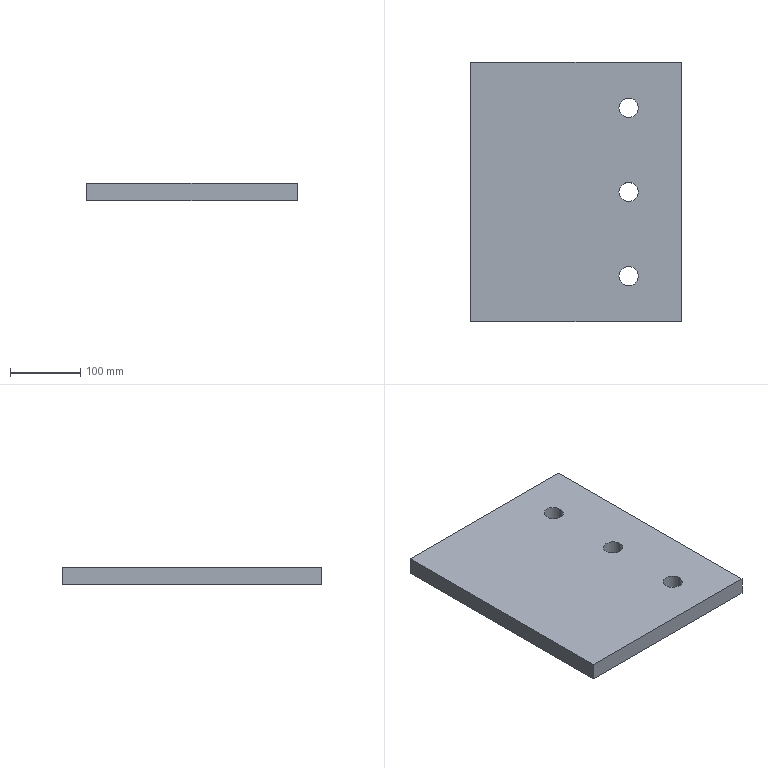Part | SolidWorks | features Extrusion 1 | 1 solid | 12 faces | box 300 x 370 x 25 mm | volume 2730453 mm3 | cylinder 6 | plane 6 | commonest cylinder face diameters 27.5 x6
STEP:
#1=CARTESIAN_POINT('',(211.25,65.,25.));
#2=VERTEX_POINT('',#1);
#3=CARTESIAN_POINT('',(238.75,65.,25.));
#4=VERTEX_POINT('',#3);
#5=CARTESIAN_POINT('',(225.,65.,25.));
#6=DIRECTION('',(0.,0.,1.));
#7=DIRECTION('',(1.,0.,0.));
#8=AXIS2_PLACEMENT_3D('',#5,#6,#7);
#9=CIRCLE('',#8,13.75);
#10=EDGE_CURVE('',#2,#4,#9,.T.);
#11=ORIENTED_EDGE('',*,*,#10,.T.);
#12=CARTESIAN_POINT('',(238.75,65.,0.));
#13=VERTEX_POINT('',#12);
#14=CARTESIAN_POINT('',(238.75,65.,25.));
#15=DIRECTION('',(0.,0.,-1.));
#16=VECTOR('',#15,1000.);
#17=LINE('',#14,#16);
#18=EDGE_CURVE('',#4,#13,#17,.T.);
#19=ORIENTED_EDGE('',*,*,#18,.T.);
#20=CARTESIAN_POINT('',(211.25,65.,0.));
#21=VERTEX_POINT('',#20);
#22=CARTESIAN_POINT('',(225.,65.,0.));
#23=DIRECTION('',(0.,0.,1.));
#24=DIRECTION('',(1.,0.,0.));
#25=AXIS2_PLACEMENT_3D('',#22,#23,#24);
#26=CIRCLE('',#25,13.75);
#27=EDGE_CURVE('',#21,#13,#26,.T.);
#28=ORIENTED_EDGE('',*,*,#27,.F.);
#29=CARTESIAN_POINT('',(211.25,65.,25.));
#30=DIRECTION('',(0.,0.,-1.));
#31=VECTOR('',#30,1000.);
#32=LINE('',#29,#31);
#33=EDGE_CURVE('',#2,#21,#32,.T.);
#34=ORIENTED_EDGE('',*,*,#33,.F.);
#35=EDGE_LOOP('',(#11,#19,#28,#34));
#36=FACE_OUTER_BOUND('',#35,.T.);
#37=CARTESIAN_POINT('',(225.,65.,25.));
#38=DIRECTION('',(0.,0.,-1.));
#39=DIRECTION('',(-1.,0.,0.));
#40=AXIS2_PLACEMENT_3D('',#37,#38,#39);
#41=CYLINDRICAL_SURFACE('',#40,13.75);
#42=ADVANCED_FACE('',(#36),#41,.F.);
#43=CARTESIAN_POINT('',(211.25,185.,25.));
#44=VERTEX_POINT('',#43);
#45=CARTESIAN_POINT('',(238.75,185.,25.));
#46=VERTEX_POINT('',#45);
#47=CARTESIAN_POINT('',(225.,185.,25.));
#48=DIRECTION('',(0.,0.,1.));
#49=DIRECTION('',(1.,0.,0.));
#50=AXIS2_PLACEMENT_3D('',#47,#48,#49);
#51=CIRCLE('',#50,13.75);
#52=EDGE_CURVE('',#44,#46,#51,.T.);
#53=ORIENTED_EDGE('',*,*,#52,.T.);
#54=CARTESIAN_POINT('',(238.75,185.,0.));
#55=VERTEX_POINT('',#54);
#56=CARTESIAN_POINT('',(238.75,185.,25.));
#57=DIRECTION('',(0.,0.,-1.));
#58=VECTOR('',#57,1000.);
#59=LINE('',#56,#58);
#60=EDGE_CURVE('',#46,#55,#59,.T.);
#61=ORIENTED_EDGE('',*,*,#60,.T.);
#62=CARTESIAN_POINT('',(211.25,185.,0.));
#63=VERTEX_POINT('',#62);
#64=CARTESIAN_POINT('',(225.,185.,0.));
#65=DIRECTION('',(0.,0.,1.));
#66=DIRECTION('',(1.,0.,0.));
#67=AXIS2_PLACEMENT_3D('',#64,#65,#66);
#68=CIRCLE('',#67,13.75);
#69=EDGE_CURVE('',#63,#55,#68,.T.);
#70=ORIENTED_EDGE('',*,*,#69,.F.);
#71=CARTESIAN_POINT('',(211.25,185.,25.));
#72=DIRECTION('',(0.,0.,-1.));
#73=VECTOR('',#72,1000.);
#74=LINE('',#71,#73);
#75=EDGE_CURVE('',#44,#63,#74,.T.);
#76=ORIENTED_EDGE('',*,*,#75,.F.);
#77=EDGE_LOOP('',(#53,#61,#70,#76));
#78=FACE_OUTER_BOUND('',#77,.T.);
#79=CARTESIAN_POINT('',(225.,185.,25.));
#80=DIRECTION('',(0.,0.,-1.));
#81=DIRECTION('',(-1.,0.,0.));
#82=AXIS2_PLACEMENT_3D('',#79,#80,#81);
#83=CYLINDRICAL_SURFACE('',#82,13.75);
#84=ADVANCED_FACE('',(#78),#83,.F.);
#85=CARTESIAN_POINT('',(211.25,305.,25.));
#86=VERTEX_POINT('',#85);
#87=CARTESIAN_POINT('',(238.75,305.,25.));
#88=VERTEX_POINT('',#87);
#89=CARTESIAN_POINT('',(225.,305.,25.));
#90=DIRECTION('',(0.,0.,1.));
#91=DIRECTION('',(1.,0.,0.));
#92=AXIS2_PLACEMENT_3D('',#89,#90,#91);
#93=CIRCLE('',#92,13.75);
#94=EDGE_CURVE('',#86,#88,#93,.T.);
#95=ORIENTED_EDGE('',*,*,#94,.T.);
#96=CARTESIAN_POINT('',(238.75,305.,0.));
#97=VERTEX_POINT('',#96);
#98=CARTESIAN_POINT('',(238.75,305.,25.));
#99=DIRECTION('',(0.,0.,-1.));
#100=VECTOR('',#99,1000.);
#101=LINE('',#98,#100);
#102=EDGE_CURVE('',#88,#97,#101,.T.);
#103=ORIENTED_EDGE('',*,*,#102,.T.);
#104=CARTESIAN_POINT('',(211.25,305.,0.));
#105=VERTEX_POINT('',#104);
#106=CARTESIAN_POINT('',(225.,305.,0.));
#107=DIRECTION('',(0.,0.,1.));
#108=DIRECTION('',(1.,0.,0.));
#109=AXIS2_PLACEMENT_3D('',#106,#107,#108);
#110=CIRCLE('',#109,13.75);
#111=EDGE_CURVE('',#105,#97,#110,.T.);
#112=ORIENTED_EDGE('',*,*,#111,.F.);
#113=CARTESIAN_POINT('',(211.25,305.,25.));
#114=DIRECTION('',(0.,0.,-1.));
#115=VECTOR('',#114,1000.);
#116=LINE('',#113,#115);
#117=EDGE_CURVE('',#86,#105,#116,.T.);
#118=ORIENTED_EDGE('',*,*,#117,.F.);
#119=EDGE_LOOP('',(#95,#103,#112,#118));
#120=FACE_OUTER_BOUND('',#119,.T.);
#121=CARTESIAN_POINT('',(225.,305.,25.));
#122=DIRECTION('',(0.,0.,-1.));
#123=DIRECTION('',(-1.,0.,0.));
#124=AXIS2_PLACEMENT_3D('',#121,#122,#123);
#125=CYLINDRICAL_SURFACE('',#124,13.75);
#126=ADVANCED_FACE('',(#120),#125,.F.);
#127=CARTESIAN_POINT('',(0.,370.,25.));
#128=VERTEX_POINT('',#127);
#129=CARTESIAN_POINT('',(0.,0.,25.));
#130=VERTEX_POINT('',#129);
#131=CARTESIAN_POINT('',(0.,0.,25.));
#132=DIRECTION('',(0.,-1.,0.));
#133=VECTOR('',#132,1000.);
#134=LINE('',#131,#133);
#135=EDGE_CURVE('',#128,#130,#134,.T.);
#136=ORIENTED_EDGE('',*,*,#135,.T.);
#137=CARTESIAN_POINT('',(300.,0.,25.));
#138=VERTEX_POINT('',#137);
#139=CARTESIAN_POINT('',(0.,0.,25.));
#140=DIRECTION('',(1.,0.,0.));
#141=VECTOR('',#140,1000.);
#142=LINE('',#139,#141);
#143=EDGE_CURVE('',#130,#138,#142,.T.);
#144=ORIENTED_EDGE('',*,*,#143,.T.);
#145=CARTESIAN_POINT('',(300.,370.,25.));
#146=VERTEX_POINT('',#145);
#147=CARTESIAN_POINT('',(300.,0.,25.));
#148=DIRECTION('',(0.,1.,0.));
#149=VECTOR('',#148,1000.);
#150=LINE('',#147,#149);
#151=EDGE_CURVE('',#138,#146,#150,.T.);
#152=ORIENTED_EDGE('',*,*,#151,.T.);
#153=CARTESIAN_POINT('',(0.,370.,25.));
#154=DIRECTION('',(-1.,0.,0.));
#155=VECTOR('',#154,1000.);
#156=LINE('',#153,#155);
#157=EDGE_CURVE('',#146,#128,#156,.T.);
#158=ORIENTED_EDGE('',*,*,#157,.T.);
#159=EDGE_LOOP('',(#136,#144,#152,#158));
#160=FACE_OUTER_BOUND('',#159,.T.);
#161=ORIENTED_EDGE('',*,*,#94,.F.);
#162=CARTESIAN_POINT('',(225.,305.,25.));
#163=DIRECTION('',(0.,0.,1.));
#164=DIRECTION('',(1.,0.,0.));
#165=AXIS2_PLACEMENT_3D('',#162,#163,#164);
#166=CIRCLE('',#165,13.75);
#167=EDGE_CURVE('',#88,#86,#166,.T.);
#168=ORIENTED_EDGE('',*,*,#167,.F.);
#169=EDGE_LOOP('',(#161,#168));
#170=FACE_BOUND('',#169,.T.);
#171=ORIENTED_EDGE('',*,*,#52,.F.);
#172=CARTESIAN_POINT('',(225.,185.,25.));
#173=DIRECTION('',(0.,0.,1.));
#174=DIRECTION('',(1.,0.,0.));
#175=AXIS2_PLACEMENT_3D('',#172,#173,#174);
#176=CIRCLE('',#175,13.75);
#177=EDGE_CURVE('',#46,#44,#176,.T.);
#178=ORIENTED_EDGE('',*,*,#177,.F.);
#179=EDGE_LOOP('',(#171,#178));
#180=FACE_BOUND('',#179,.T.);
#181=ORIENTED_EDGE('',*,*,#10,.F.);
#182=CARTESIAN_POINT('',(225.,65.,25.));
#183=DIRECTION('',(0.,0.,1.));
#184=DIRECTION('',(1.,0.,0.));
#185=AXIS2_PLACEMENT_3D('',#182,#183,#184);
#186=CIRCLE('',#185,13.75);
#187=EDGE_CURVE('',#4,#2,#186,.T.);
#188=ORIENTED_EDGE('',*,*,#187,.F.);
#189=EDGE_LOOP('',(#181,#188));
#190=FACE_BOUND('',#189,.T.);
#191=CARTESIAN_POINT('',(0.,0.,25.));
#192=DIRECTION('',(0.,0.,-1.));
#193=DIRECTION('',(-1.,0.,0.));
#194=AXIS2_PLACEMENT_3D('',#191,#192,#193);
#195=PLANE('',#194);
#196=ADVANCED_FACE('',(#160,#170,#180,#190),#195,.F.);
#197=ORIENTED_EDGE('',*,*,#69,.T.);
#198=CARTESIAN_POINT('',(225.,185.,0.));
#199=DIRECTION('',(0.,0.,1.));
#200=DIRECTION('',(1.,0.,0.));
#201=AXIS2_PLACEMENT_3D('',#198,#199,#200);
#202=CIRCLE('',#201,13.75);
#203=EDGE_CURVE('',#55,#63,#202,.T.);
#204=ORIENTED_EDGE('',*,*,#203,.T.);
#205=EDGE_LOOP('',(#197,#204));
#206=FACE_BOUND('',#205,.T.);
#207=CARTESIAN_POINT('',(0.,370.,0.));
#208=VERTEX_POINT('',#207);
#209=CARTESIAN_POINT('',(0.,0.,0.));
#210=VERTEX_POINT('',#209);
#211=CARTESIAN_POINT('',(0.,0.,0.));
#212=DIRECTION('',(0.,-1.,0.));
#213=VECTOR('',#212,1000.);
#214=LINE('',#211,#213);
#215=EDGE_CURVE('',#208,#210,#214,.T.);
#216=ORIENTED_EDGE('',*,*,#215,.F.);
#217=CARTESIAN_POINT('',(300.,370.,0.));
#218=VERTEX_POINT('',#217);
#219=CARTESIAN_POINT('',(0.,370.,0.));
#220=DIRECTION('',(-1.,0.,0.));
#221=VECTOR('',#220,1000.);
#222=LINE('',#219,#221);
#223=EDGE_CURVE('',#218,#208,#222,.T.);
#224=ORIENTED_EDGE('',*,*,#223,.F.);
#225=CARTESIAN_POINT('',(300.,0.,0.));
#226=VERTEX_POINT('',#225);
#227=CARTESIAN_POINT('',(300.,0.,0.));
#228=DIRECTION('',(0.,1.,0.));
#229=VECTOR('',#228,1000.);
#230=LINE('',#227,#229);
#231=EDGE_CURVE('',#226,#218,#230,.T.);
#232=ORIENTED_EDGE('',*,*,#231,.F.);
#233=CARTESIAN_POINT('',(0.,0.,0.));
#234=DIRECTION('',(1.,0.,0.));
#235=VECTOR('',#234,1000.);
#236=LINE('',#233,#235);
#237=EDGE_CURVE('',#210,#226,#236,.T.);
#238=ORIENTED_EDGE('',*,*,#237,.F.);
#239=EDGE_LOOP('',(#216,#224,#232,#238));
#240=FACE_OUTER_BOUND('',#239,.T.);
#241=ORIENTED_EDGE('',*,*,#111,.T.);
#242=CARTESIAN_POINT('',(225.,305.,0.));
#243=DIRECTION('',(0.,0.,1.));
#244=DIRECTION('',(1.,0.,0.));
#245=AXIS2_PLACEMENT_3D('',#242,#243,#244);
#246=CIRCLE('',#245,13.75);
#247=EDGE_CURVE('',#97,#105,#246,.T.);
#248=ORIENTED_EDGE('',*,*,#247,.T.);
#249=EDGE_LOOP('',(#241,#248));
#250=FACE_BOUND('',#249,.T.);
#251=ORIENTED_EDGE('',*,*,#27,.T.);
#252=CARTESIAN_POINT('',(225.,65.,0.));
#253=DIRECTION('',(0.,0.,1.));
#254=DIRECTION('',(1.,0.,0.));
#255=AXIS2_PLACEMENT_3D('',#252,#253,#254);
#256=CIRCLE('',#255,13.75);
#257=EDGE_CURVE('',#13,#21,#256,.T.);
#258=ORIENTED_EDGE('',*,*,#257,.T.);
#259=EDGE_LOOP('',(#251,#258));
#260=FACE_BOUND('',#259,.T.);
#261=CARTESIAN_POINT('',(0.,0.,0.));
#262=DIRECTION('',(0.,0.,-1.));
#263=DIRECTION('',(-1.,0.,0.));
#264=AXIS2_PLACEMENT_3D('',#261,#262,#263);
#265=PLANE('',#264);
#266=ADVANCED_FACE('',(#206,#240,#250,#260),#265,.T.);
#267=ORIENTED_EDGE('',*,*,#215,.T.);
#268=CARTESIAN_POINT('',(0.,0.,25.));
#269=DIRECTION('',(0.,0.,-1.));
#270=VECTOR('',#269,1000.);
#271=LINE('',#268,#270);
#272=EDGE_CURVE('',#130,#210,#271,.T.);
#273=ORIENTED_EDGE('',*,*,#272,.F.);
#274=ORIENTED_EDGE('',*,*,#135,.F.);
#275=CARTESIAN_POINT('',(0.,370.,25.));
#276=DIRECTION('',(0.,0.,-1.));
#277=VECTOR('',#276,1000.);
#278=LINE('',#275,#277);
#279=EDGE_CURVE('',#128,#208,#278,.T.);
#280=ORIENTED_EDGE('',*,*,#279,.T.);
#281=EDGE_LOOP('',(#267,#273,#274,#280));
#282=FACE_OUTER_BOUND('',#281,.T.);
#283=CARTESIAN_POINT('',(0.,0.,25.));
#284=DIRECTION('',(1.,0.,0.));
#285=DIRECTION('',(0.,0.,-1.));
#286=AXIS2_PLACEMENT_3D('',#283,#284,#285);
#287=PLANE('',#286);
#288=ADVANCED_FACE('',(#282),#287,.F.);
#289=ORIENTED_EDGE('',*,*,#237,.T.);
#290=CARTESIAN_POINT('',(300.,0.,25.));
#291=DIRECTION('',(0.,0.,-1.));
#292=VECTOR('',#291,1000.);
#293=LINE('',#290,#292);
#294=EDGE_CURVE('',#138,#226,#293,.T.);
#295=ORIENTED_EDGE('',*,*,#294,.F.);
#296=ORIENTED_EDGE('',*,*,#143,.F.);
#297=ORIENTED_EDGE('',*,*,#272,.T.);
#298=EDGE_LOOP('',(#289,#295,#296,#297));
#299=FACE_OUTER_BOUND('',#298,.T.);
#300=CARTESIAN_POINT('',(0.,0.,25.));
#301=DIRECTION('',(0.,1.,0.));
#302=DIRECTION('',(0.,0.,1.));
#303=AXIS2_PLACEMENT_3D('',#300,#301,#302);
#304=PLANE('',#303);
#305=ADVANCED_FACE('',(#299),#304,.F.);
#306=ORIENTED_EDGE('',*,*,#231,.T.);
#307=CARTESIAN_POINT('',(300.,370.,25.));
#308=DIRECTION('',(0.,0.,-1.));
#309=VECTOR('',#308,1000.);
#310=LINE('',#307,#309);
#311=EDGE_CURVE('',#146,#218,#310,.T.);
#312=ORIENTED_EDGE('',*,*,#311,.F.);
#313=ORIENTED_EDGE('',*,*,#151,.F.);
#314=ORIENTED_EDGE('',*,*,#294,.T.);
#315=EDGE_LOOP('',(#306,#312,#313,#314));
#316=FACE_OUTER_BOUND('',#315,.T.);
#317=CARTESIAN_POINT('',(300.,0.,25.));
#318=DIRECTION('',(-1.,0.,0.));
#319=DIRECTION('',(0.,0.,1.));
#320=AXIS2_PLACEMENT_3D('',#317,#318,#319);
#321=PLANE('',#320);
#322=ADVANCED_FACE('',(#316),#321,.F.);
#323=ORIENTED_EDGE('',*,*,#223,.T.);
#324=ORIENTED_EDGE('',*,*,#279,.F.);
#325=ORIENTED_EDGE('',*,*,#157,.F.);
#326=ORIENTED_EDGE('',*,*,#311,.T.);
#327=EDGE_LOOP('',(#323,#324,#325,#326));
#328=FACE_OUTER_BOUND('',#327,.T.);
#329=CARTESIAN_POINT('',(0.,370.,25.));
#330=DIRECTION('',(0.,-1.,0.));
#331=DIRECTION('',(0.,0.,-1.));
#332=AXIS2_PLACEMENT_3D('',#329,#330,#331);
#333=PLANE('',#332);
#334=ADVANCED_FACE('',(#328),#333,.F.);
#335=ORIENTED_EDGE('',*,*,#102,.F.);
#336=ORIENTED_EDGE('',*,*,#167,.T.);
#337=ORIENTED_EDGE('',*,*,#117,.T.);
#338=ORIENTED_EDGE('',*,*,#247,.F.);
#339=EDGE_LOOP('',(#335,#336,#337,#338));
#340=FACE_OUTER_BOUND('',#339,.T.);
#341=CARTESIAN_POINT('',(225.,305.,25.));
#342=DIRECTION('',(0.,0.,-1.));
#343=DIRECTION('',(-1.,0.,0.));
#344=AXIS2_PLACEMENT_3D('',#341,#342,#343);
#345=CYLINDRICAL_SURFACE('',#344,13.75);
#346=ADVANCED_FACE('',(#340),#345,.F.);
#347=ORIENTED_EDGE('',*,*,#60,.F.);
#348=ORIENTED_EDGE('',*,*,#177,.T.);
#349=ORIENTED_EDGE('',*,*,#75,.T.);
#350=ORIENTED_EDGE('',*,*,#203,.F.);
#351=EDGE_LOOP('',(#347,#348,#349,#350));
#352=FACE_OUTER_BOUND('',#351,.T.);
#353=CARTESIAN_POINT('',(225.,185.,25.));
#354=DIRECTION('',(0.,0.,-1.));
#355=DIRECTION('',(-1.,0.,0.));
#356=AXIS2_PLACEMENT_3D('',#353,#354,#355);
#357=CYLINDRICAL_SURFACE('',#356,13.75);
#358=ADVANCED_FACE('',(#352),#357,.F.);
#359=ORIENTED_EDGE('',*,*,#18,.F.);
#360=ORIENTED_EDGE('',*,*,#187,.T.);
#361=ORIENTED_EDGE('',*,*,#33,.T.);
#362=ORIENTED_EDGE('',*,*,#257,.F.);
#363=EDGE_LOOP('',(#359,#360,#361,#362));
#364=FACE_OUTER_BOUND('',#363,.T.);
#365=CARTESIAN_POINT('',(225.,65.,25.));
#366=DIRECTION('',(0.,0.,-1.));
#367=DIRECTION('',(-1.,0.,0.));
#368=AXIS2_PLACEMENT_3D('',#365,#366,#367);
#369=CYLINDRICAL_SURFACE('',#368,13.75);
#370=ADVANCED_FACE('',(#364),#369,.F.);
#371=CLOSED_SHELL('',(#42,#84,#126,#196,#266,#288,#305,#322,#334,#346,#358,#370));
#372=MANIFOLD_SOLID_BREP('',#371);
#373=CARTESIAN_POINT('',(0.,0.,0.));
#374=DIRECTION('',(0.,0.,1.));
#375=DIRECTION('',(1.,0.,0.));
#376=AXIS2_PLACEMENT_3D('',#373,#374,#375);
#377=(LENGTH_UNIT()NAMED_UNIT(*)SI_UNIT(.MILLI.,.METRE.));
#378=UNCERTAINTY_MEASURE_WITH_UNIT(LENGTH_MEASURE(0.00001),#377,'','');
#379=(NAMED_UNIT(*)PLANE_ANGLE_UNIT()SI_UNIT($,.RADIAN.));
#380=(NAMED_UNIT(*)SI_UNIT($,.STERADIAN.)SOLID_ANGLE_UNIT());
#381=(GEOMETRIC_REPRESENTATION_CONTEXT(3)GLOBAL_UNCERTAINTY_ASSIGNED_CONTEXT((#378))GLOBAL_UNIT_ASSIGNED_CONTEXT((#377,#379,#380))REPRESENTATION_CONTEXT('',''));
#382=ADVANCED_BREP_SHAPE_REPRESENTATION('',(#372,#376),#381);